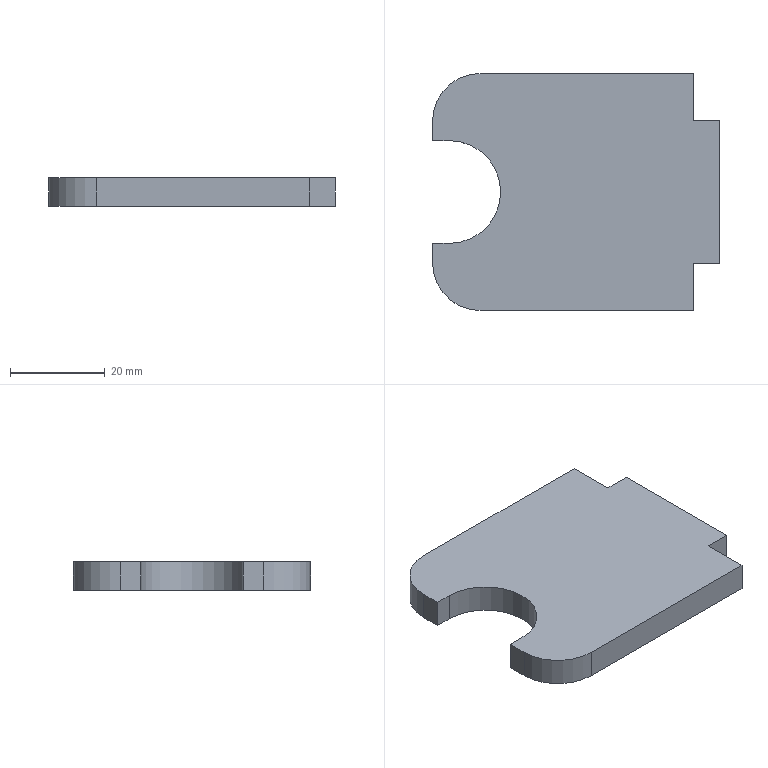Part | SolidWorks | features FlatPattern 1, SMBaseFlange 1, SheetMetal 1 | 1 solid | 16 faces | box 60.5 x 50 x 6 mm | volume 15667 mm3 | plane 13 | cylinder 3 | commonest cylinder face diameters 20 x2 21.7 x1
STEP:
#1=CARTESIAN_POINT('',(-93.75,45.198,0.));
#2=VERTEX_POINT('',#1);
#3=CARTESIAN_POINT('',(-93.75,23.498,0.));
#4=VERTEX_POINT('',#3);
#5=CARTESIAN_POINT('',(-93.75,34.348,0.));
#6=DIRECTION('',(0.,0.,-1.));
#7=DIRECTION('',(1.,0.,0.));
#8=AXIS2_PLACEMENT_3D('',#5,#6,#7);
#9=CIRCLE('',#8,10.85);
#10=EDGE_CURVE('',#2,#4,#9,.T.);
#11=ORIENTED_EDGE('',*,*,#10,.T.);
#12=CARTESIAN_POINT('',(-93.75,23.498,6.));
#13=VERTEX_POINT('',#12);
#14=CARTESIAN_POINT('',(-93.75,23.498,6.));
#15=DIRECTION('',(0.,0.,-1.));
#16=VECTOR('',#15,1000.);
#17=LINE('',#14,#16);
#18=EDGE_CURVE('',#13,#4,#17,.T.);
#19=ORIENTED_EDGE('',*,*,#18,.F.);
#20=CARTESIAN_POINT('',(-93.75,45.198,6.));
#21=VERTEX_POINT('',#20);
#22=CARTESIAN_POINT('',(-93.75,34.348,6.));
#23=DIRECTION('',(0.,0.,-1.));
#24=DIRECTION('',(1.,0.,0.));
#25=AXIS2_PLACEMENT_3D('',#22,#23,#24);
#26=CIRCLE('',#25,10.85);
#27=EDGE_CURVE('',#21,#13,#26,.T.);
#28=ORIENTED_EDGE('',*,*,#27,.F.);
#29=CARTESIAN_POINT('',(-93.75,45.198,6.));
#30=DIRECTION('',(0.,0.,-1.));
#31=VECTOR('',#30,1000.);
#32=LINE('',#29,#31);
#33=EDGE_CURVE('',#21,#2,#32,.T.);
#34=ORIENTED_EDGE('',*,*,#33,.T.);
#35=EDGE_LOOP('',(#11,#19,#28,#34));
#36=FACE_OUTER_BOUND('',#35,.T.);
#37=CARTESIAN_POINT('',(-93.75,34.348,6.));
#38=DIRECTION('',(0.,0.,-1.));
#39=DIRECTION('',(-1.,0.,0.));
#40=AXIS2_PLACEMENT_3D('',#37,#38,#39);
#41=CYLINDRICAL_SURFACE('',#40,10.85);
#42=ADVANCED_FACE('',(#36),#41,.F.);
#43=CARTESIAN_POINT('',(-97.25,23.498,0.));
#44=VERTEX_POINT('',#43);
#45=CARTESIAN_POINT('',(-93.75,23.498,0.));
#46=DIRECTION('',(-1.,0.,0.));
#47=VECTOR('',#46,1000.);
#48=LINE('',#45,#47);
#49=EDGE_CURVE('',#4,#44,#48,.T.);
#50=ORIENTED_EDGE('',*,*,#49,.T.);
#51=CARTESIAN_POINT('',(-97.25,23.498,6.));
#52=VERTEX_POINT('',#51);
#53=CARTESIAN_POINT('',(-97.25,23.498,6.));
#54=DIRECTION('',(0.,0.,-1.));
#55=VECTOR('',#54,1000.);
#56=LINE('',#53,#55);
#57=EDGE_CURVE('',#52,#44,#56,.T.);
#58=ORIENTED_EDGE('',*,*,#57,.F.);
#59=CARTESIAN_POINT('',(-93.75,23.498,6.));
#60=DIRECTION('',(-1.,0.,0.));
#61=VECTOR('',#60,1000.);
#62=LINE('',#59,#61);
#63=EDGE_CURVE('',#13,#52,#62,.T.);
#64=ORIENTED_EDGE('',*,*,#63,.F.);
#65=ORIENTED_EDGE('',*,*,#18,.T.);
#66=EDGE_LOOP('',(#50,#58,#64,#65));
#67=FACE_OUTER_BOUND('',#66,.T.);
#68=CARTESIAN_POINT('',(-93.75,23.498,6.));
#69=DIRECTION('',(0.,-1.,0.));
#70=DIRECTION('',(0.,0.,-1.));
#71=AXIS2_PLACEMENT_3D('',#68,#69,#70);
#72=PLANE('',#71);
#73=ADVANCED_FACE('',(#67),#72,.F.);
#74=CARTESIAN_POINT('',(-97.25,19.348,0.));
#75=VERTEX_POINT('',#74);
#76=CARTESIAN_POINT('',(-97.25,23.498,0.));
#77=DIRECTION('',(0.,-1.,0.));
#78=VECTOR('',#77,1000.);
#79=LINE('',#76,#78);
#80=EDGE_CURVE('',#44,#75,#79,.T.);
#81=ORIENTED_EDGE('',*,*,#80,.T.);
#82=CARTESIAN_POINT('',(-97.25,19.348,6.));
#83=VERTEX_POINT('',#82);
#84=CARTESIAN_POINT('',(-97.25,19.348,6.));
#85=DIRECTION('',(0.,0.,-1.));
#86=VECTOR('',#85,1000.);
#87=LINE('',#84,#86);
#88=EDGE_CURVE('',#83,#75,#87,.T.);
#89=ORIENTED_EDGE('',*,*,#88,.F.);
#90=CARTESIAN_POINT('',(-97.25,23.498,6.));
#91=DIRECTION('',(0.,-1.,0.));
#92=VECTOR('',#91,1000.);
#93=LINE('',#90,#92);
#94=EDGE_CURVE('',#52,#83,#93,.T.);
#95=ORIENTED_EDGE('',*,*,#94,.F.);
#96=ORIENTED_EDGE('',*,*,#57,.T.);
#97=EDGE_LOOP('',(#81,#89,#95,#96));
#98=FACE_OUTER_BOUND('',#97,.T.);
#99=CARTESIAN_POINT('',(-97.25,23.498,6.));
#100=DIRECTION('',(1.,0.,0.));
#101=DIRECTION('',(0.,1.,0.));
#102=AXIS2_PLACEMENT_3D('',#99,#100,#101);
#103=PLANE('',#102);
#104=ADVANCED_FACE('',(#98),#103,.F.);
#105=CARTESIAN_POINT('',(-87.25,9.348,0.));
#106=VERTEX_POINT('',#105);
#107=CARTESIAN_POINT('',(-87.25,19.348,0.));
#108=DIRECTION('',(0.,0.,1.));
#109=DIRECTION('',(1.,0.,0.));
#110=AXIS2_PLACEMENT_3D('',#107,#108,#109);
#111=CIRCLE('',#110,10.);
#112=EDGE_CURVE('',#75,#106,#111,.T.);
#113=ORIENTED_EDGE('',*,*,#112,.T.);
#114=CARTESIAN_POINT('',(-87.25,9.348,6.));
#115=VERTEX_POINT('',#114);
#116=CARTESIAN_POINT('',(-87.25,9.348,6.));
#117=DIRECTION('',(0.,0.,-1.));
#118=VECTOR('',#117,1000.);
#119=LINE('',#116,#118);
#120=EDGE_CURVE('',#115,#106,#119,.T.);
#121=ORIENTED_EDGE('',*,*,#120,.F.);
#122=CARTESIAN_POINT('',(-87.25,19.348,6.));
#123=DIRECTION('',(0.,0.,1.));
#124=DIRECTION('',(1.,0.,0.));
#125=AXIS2_PLACEMENT_3D('',#122,#123,#124);
#126=CIRCLE('',#125,10.);
#127=EDGE_CURVE('',#83,#115,#126,.T.);
#128=ORIENTED_EDGE('',*,*,#127,.F.);
#129=ORIENTED_EDGE('',*,*,#88,.T.);
#130=EDGE_LOOP('',(#113,#121,#128,#129));
#131=FACE_OUTER_BOUND('',#130,.T.);
#132=CARTESIAN_POINT('',(-87.25,19.348,6.));
#133=DIRECTION('',(0.,0.,-1.));
#134=DIRECTION('',(-1.,0.,0.));
#135=AXIS2_PLACEMENT_3D('',#132,#133,#134);
#136=CYLINDRICAL_SURFACE('',#135,10.);
#137=ADVANCED_FACE('',(#131),#136,.T.);
#138=CARTESIAN_POINT('',(-42.25,9.348,0.));
#139=VERTEX_POINT('',#138);
#140=CARTESIAN_POINT('',(-87.25,9.348,0.));
#141=DIRECTION('',(1.,0.,0.));
#142=VECTOR('',#141,1000.);
#143=LINE('',#140,#142);
#144=EDGE_CURVE('',#106,#139,#143,.T.);
#145=ORIENTED_EDGE('',*,*,#144,.T.);
#146=CARTESIAN_POINT('',(-42.25,9.348,6.));
#147=VERTEX_POINT('',#146);
#148=CARTESIAN_POINT('',(-42.25,9.348,6.));
#149=DIRECTION('',(0.,0.,-1.));
#150=VECTOR('',#149,1000.);
#151=LINE('',#148,#150);
#152=EDGE_CURVE('',#147,#139,#151,.T.);
#153=ORIENTED_EDGE('',*,*,#152,.F.);
#154=CARTESIAN_POINT('',(-87.25,9.348,6.));
#155=DIRECTION('',(1.,0.,0.));
#156=VECTOR('',#155,1000.);
#157=LINE('',#154,#156);
#158=EDGE_CURVE('',#115,#147,#157,.T.);
#159=ORIENTED_EDGE('',*,*,#158,.F.);
#160=ORIENTED_EDGE('',*,*,#120,.T.);
#161=EDGE_LOOP('',(#145,#153,#159,#160));
#162=FACE_OUTER_BOUND('',#161,.T.);
#163=CARTESIAN_POINT('',(-87.25,9.348,6.));
#164=DIRECTION('',(0.,1.,0.));
#165=DIRECTION('',(-1.,0.,0.));
#166=AXIS2_PLACEMENT_3D('',#163,#164,#165);
#167=PLANE('',#166);
#168=ADVANCED_FACE('',(#162),#167,.F.);
#169=CARTESIAN_POINT('',(-42.25,19.348,0.));
#170=VERTEX_POINT('',#169);
#171=CARTESIAN_POINT('',(-42.25,9.348,0.));
#172=DIRECTION('',(0.,1.,0.));
#173=VECTOR('',#172,1000.);
#174=LINE('',#171,#173);
#175=EDGE_CURVE('',#139,#170,#174,.T.);
#176=ORIENTED_EDGE('',*,*,#175,.T.);
#177=CARTESIAN_POINT('',(-42.25,19.348,6.));
#178=VERTEX_POINT('',#177);
#179=CARTESIAN_POINT('',(-42.25,19.348,6.));
#180=DIRECTION('',(0.,0.,-1.));
#181=VECTOR('',#180,1000.);
#182=LINE('',#179,#181);
#183=EDGE_CURVE('',#178,#170,#182,.T.);
#184=ORIENTED_EDGE('',*,*,#183,.F.);
#185=CARTESIAN_POINT('',(-42.25,9.348,6.));
#186=DIRECTION('',(0.,1.,0.));
#187=VECTOR('',#186,1000.);
#188=LINE('',#185,#187);
#189=EDGE_CURVE('',#147,#178,#188,.T.);
#190=ORIENTED_EDGE('',*,*,#189,.F.);
#191=ORIENTED_EDGE('',*,*,#152,.T.);
#192=EDGE_LOOP('',(#176,#184,#190,#191));
#193=FACE_OUTER_BOUND('',#192,.T.);
#194=CARTESIAN_POINT('',(-42.25,9.348,6.));
#195=DIRECTION('',(-1.,0.,0.));
#196=DIRECTION('',(0.,0.,1.));
#197=AXIS2_PLACEMENT_3D('',#194,#195,#196);
#198=PLANE('',#197);
#199=ADVANCED_FACE('',(#193),#198,.F.);
#200=CARTESIAN_POINT('',(-36.75,19.348,0.));
#201=VERTEX_POINT('',#200);
#202=CARTESIAN_POINT('',(-42.25,19.348,0.));
#203=DIRECTION('',(1.,0.,0.));
#204=VECTOR('',#203,1000.);
#205=LINE('',#202,#204);
#206=EDGE_CURVE('',#170,#201,#205,.T.);
#207=ORIENTED_EDGE('',*,*,#206,.T.);
#208=CARTESIAN_POINT('',(-36.75,19.348,6.));
#209=VERTEX_POINT('',#208);
#210=CARTESIAN_POINT('',(-36.75,19.348,6.));
#211=DIRECTION('',(0.,0.,-1.));
#212=VECTOR('',#211,1000.);
#213=LINE('',#210,#212);
#214=EDGE_CURVE('',#209,#201,#213,.T.);
#215=ORIENTED_EDGE('',*,*,#214,.F.);
#216=CARTESIAN_POINT('',(-42.25,19.348,6.));
#217=DIRECTION('',(1.,0.,0.));
#218=VECTOR('',#217,1000.);
#219=LINE('',#216,#218);
#220=EDGE_CURVE('',#178,#209,#219,.T.);
#221=ORIENTED_EDGE('',*,*,#220,.F.);
#222=ORIENTED_EDGE('',*,*,#183,.T.);
#223=EDGE_LOOP('',(#207,#215,#221,#222));
#224=FACE_OUTER_BOUND('',#223,.T.);
#225=CARTESIAN_POINT('',(-42.25,19.348,6.));
#226=DIRECTION('',(0.,1.,0.));
#227=DIRECTION('',(-1.,0.,0.));
#228=AXIS2_PLACEMENT_3D('',#225,#226,#227);
#229=PLANE('',#228);
#230=ADVANCED_FACE('',(#224),#229,.F.);
#231=CARTESIAN_POINT('',(-36.75,49.348,0.));
#232=VERTEX_POINT('',#231);
#233=CARTESIAN_POINT('',(-36.75,19.348,0.));
#234=DIRECTION('',(0.,1.,0.));
#235=VECTOR('',#234,1000.);
#236=LINE('',#233,#235);
#237=EDGE_CURVE('',#201,#232,#236,.T.);
#238=ORIENTED_EDGE('',*,*,#237,.T.);
#239=CARTESIAN_POINT('',(-36.75,49.348,6.));
#240=VERTEX_POINT('',#239);
#241=CARTESIAN_POINT('',(-36.75,49.348,6.));
#242=DIRECTION('',(0.,0.,-1.));
#243=VECTOR('',#242,1000.);
#244=LINE('',#241,#243);
#245=EDGE_CURVE('',#240,#232,#244,.T.);
#246=ORIENTED_EDGE('',*,*,#245,.F.);
#247=CARTESIAN_POINT('',(-36.75,19.348,6.));
#248=DIRECTION('',(0.,1.,0.));
#249=VECTOR('',#248,1000.);
#250=LINE('',#247,#249);
#251=EDGE_CURVE('',#209,#240,#250,.T.);
#252=ORIENTED_EDGE('',*,*,#251,.F.);
#253=ORIENTED_EDGE('',*,*,#214,.T.);
#254=EDGE_LOOP('',(#238,#246,#252,#253));
#255=FACE_OUTER_BOUND('',#254,.T.);
#256=CARTESIAN_POINT('',(-36.75,19.348,6.));
#257=DIRECTION('',(-1.,0.,0.));
#258=DIRECTION('',(0.,0.,1.));
#259=AXIS2_PLACEMENT_3D('',#256,#257,#258);
#260=PLANE('',#259);
#261=ADVANCED_FACE('',(#255),#260,.F.);
#262=CARTESIAN_POINT('',(-42.25,49.348,0.));
#263=VERTEX_POINT('',#262);
#264=CARTESIAN_POINT('',(-36.75,49.348,0.));
#265=DIRECTION('',(-1.,0.,0.));
#266=VECTOR('',#265,1000.);
#267=LINE('',#264,#266);
#268=EDGE_CURVE('',#232,#263,#267,.T.);
#269=ORIENTED_EDGE('',*,*,#268,.T.);
#270=CARTESIAN_POINT('',(-42.25,49.348,6.));
#271=VERTEX_POINT('',#270);
#272=CARTESIAN_POINT('',(-42.25,49.348,6.));
#273=DIRECTION('',(0.,0.,-1.));
#274=VECTOR('',#273,1000.);
#275=LINE('',#272,#274);
#276=EDGE_CURVE('',#271,#263,#275,.T.);
#277=ORIENTED_EDGE('',*,*,#276,.F.);
#278=CARTESIAN_POINT('',(-36.75,49.348,6.));
#279=DIRECTION('',(-1.,0.,0.));
#280=VECTOR('',#279,1000.);
#281=LINE('',#278,#280);
#282=EDGE_CURVE('',#240,#271,#281,.T.);
#283=ORIENTED_EDGE('',*,*,#282,.F.);
#284=ORIENTED_EDGE('',*,*,#245,.T.);
#285=EDGE_LOOP('',(#269,#277,#283,#284));
#286=FACE_OUTER_BOUND('',#285,.T.);
#287=CARTESIAN_POINT('',(-36.75,49.348,6.));
#288=DIRECTION('',(0.,-1.,0.));
#289=DIRECTION('',(1.,0.,0.));
#290=AXIS2_PLACEMENT_3D('',#287,#288,#289);
#291=PLANE('',#290);
#292=ADVANCED_FACE('',(#286),#291,.F.);
#293=CARTESIAN_POINT('',(-42.25,59.348,0.));
#294=VERTEX_POINT('',#293);
#295=CARTESIAN_POINT('',(-42.25,49.348,0.));
#296=DIRECTION('',(0.,1.,0.));
#297=VECTOR('',#296,1000.);
#298=LINE('',#295,#297);
#299=EDGE_CURVE('',#263,#294,#298,.T.);
#300=ORIENTED_EDGE('',*,*,#299,.T.);
#301=CARTESIAN_POINT('',(-42.25,59.348,6.));
#302=VERTEX_POINT('',#301);
#303=CARTESIAN_POINT('',(-42.25,59.348,6.));
#304=DIRECTION('',(0.,0.,-1.));
#305=VECTOR('',#304,1000.);
#306=LINE('',#303,#305);
#307=EDGE_CURVE('',#302,#294,#306,.T.);
#308=ORIENTED_EDGE('',*,*,#307,.F.);
#309=CARTESIAN_POINT('',(-42.25,49.348,6.));
#310=DIRECTION('',(0.,1.,0.));
#311=VECTOR('',#310,1000.);
#312=LINE('',#309,#311);
#313=EDGE_CURVE('',#271,#302,#312,.T.);
#314=ORIENTED_EDGE('',*,*,#313,.F.);
#315=ORIENTED_EDGE('',*,*,#276,.T.);
#316=EDGE_LOOP('',(#300,#308,#314,#315));
#317=FACE_OUTER_BOUND('',#316,.T.);
#318=CARTESIAN_POINT('',(-42.25,49.348,6.));
#319=DIRECTION('',(-1.,0.,0.));
#320=DIRECTION('',(0.,0.,1.));
#321=AXIS2_PLACEMENT_3D('',#318,#319,#320);
#322=PLANE('',#321);
#323=ADVANCED_FACE('',(#317),#322,.F.);
#324=CARTESIAN_POINT('',(-87.25,59.348,0.));
#325=VERTEX_POINT('',#324);
#326=CARTESIAN_POINT('',(-87.25,59.348,0.));
#327=DIRECTION('',(-1.,0.,0.));
#328=VECTOR('',#327,1000.);
#329=LINE('',#326,#328);
#330=EDGE_CURVE('',#294,#325,#329,.T.);
#331=ORIENTED_EDGE('',*,*,#330,.T.);
#332=CARTESIAN_POINT('',(-87.25,59.348,6.));
#333=VERTEX_POINT('',#332);
#334=CARTESIAN_POINT('',(-87.25,59.348,6.));
#335=DIRECTION('',(0.,0.,-1.));
#336=VECTOR('',#335,1000.);
#337=LINE('',#334,#336);
#338=EDGE_CURVE('',#333,#325,#337,.T.);
#339=ORIENTED_EDGE('',*,*,#338,.F.);
#340=CARTESIAN_POINT('',(-87.25,59.348,6.));
#341=DIRECTION('',(-1.,0.,0.));
#342=VECTOR('',#341,1000.);
#343=LINE('',#340,#342);
#344=EDGE_CURVE('',#302,#333,#343,.T.);
#345=ORIENTED_EDGE('',*,*,#344,.F.);
#346=ORIENTED_EDGE('',*,*,#307,.T.);
#347=EDGE_LOOP('',(#331,#339,#345,#346));
#348=FACE_OUTER_BOUND('',#347,.T.);
#349=CARTESIAN_POINT('',(-87.25,59.348,6.));
#350=DIRECTION('',(0.,-1.,0.));
#351=DIRECTION('',(0.,0.,-1.));
#352=AXIS2_PLACEMENT_3D('',#349,#350,#351);
#353=PLANE('',#352);
#354=ADVANCED_FACE('',(#348),#353,.F.);
#355=CARTESIAN_POINT('',(-97.25,49.348,0.));
#356=VERTEX_POINT('',#355);
#357=CARTESIAN_POINT('',(-87.25,49.348,0.));
#358=DIRECTION('',(0.,0.,1.));
#359=DIRECTION('',(-1.,0.,0.));
#360=AXIS2_PLACEMENT_3D('',#357,#358,#359);
#361=CIRCLE('',#360,10.);
#362=EDGE_CURVE('',#325,#356,#361,.T.);
#363=ORIENTED_EDGE('',*,*,#362,.T.);
#364=CARTESIAN_POINT('',(-97.25,49.348,6.));
#365=VERTEX_POINT('',#364);
#366=CARTESIAN_POINT('',(-97.25,49.348,6.));
#367=DIRECTION('',(0.,0.,-1.));
#368=VECTOR('',#367,1000.);
#369=LINE('',#366,#368);
#370=EDGE_CURVE('',#365,#356,#369,.T.);
#371=ORIENTED_EDGE('',*,*,#370,.F.);
#372=CARTESIAN_POINT('',(-87.25,49.348,6.));
#373=DIRECTION('',(0.,0.,1.));
#374=DIRECTION('',(-1.,0.,0.));
#375=AXIS2_PLACEMENT_3D('',#372,#373,#374);
#376=CIRCLE('',#375,10.);
#377=EDGE_CURVE('',#333,#365,#376,.T.);
#378=ORIENTED_EDGE('',*,*,#377,.F.);
#379=ORIENTED_EDGE('',*,*,#338,.T.);
#380=EDGE_LOOP('',(#363,#371,#378,#379));
#381=FACE_OUTER_BOUND('',#380,.T.);
#382=CARTESIAN_POINT('',(-87.25,49.348,6.));
#383=DIRECTION('',(0.,0.,-1.));
#384=DIRECTION('',(-1.,0.,0.));
#385=AXIS2_PLACEMENT_3D('',#382,#383,#384);
#386=CYLINDRICAL_SURFACE('',#385,10.);
#387=ADVANCED_FACE('',(#381),#386,.T.);
#388=CARTESIAN_POINT('',(-97.25,45.198,0.));
#389=VERTEX_POINT('',#388);
#390=CARTESIAN_POINT('',(-97.25,45.198,0.));
#391=DIRECTION('',(0.,-1.,0.));
#392=VECTOR('',#391,1000.);
#393=LINE('',#390,#392);
#394=EDGE_CURVE('',#356,#389,#393,.T.);
#395=ORIENTED_EDGE('',*,*,#394,.T.);
#396=CARTESIAN_POINT('',(-97.25,45.198,6.));
#397=VERTEX_POINT('',#396);
#398=CARTESIAN_POINT('',(-97.25,45.198,6.));
#399=DIRECTION('',(0.,0.,-1.));
#400=VECTOR('',#399,1000.);
#401=LINE('',#398,#400);
#402=EDGE_CURVE('',#397,#389,#401,.T.);
#403=ORIENTED_EDGE('',*,*,#402,.F.);
#404=CARTESIAN_POINT('',(-97.25,45.198,6.));
#405=DIRECTION('',(0.,-1.,0.));
#406=VECTOR('',#405,1000.);
#407=LINE('',#404,#406);
#408=EDGE_CURVE('',#365,#397,#407,.T.);
#409=ORIENTED_EDGE('',*,*,#408,.F.);
#410=ORIENTED_EDGE('',*,*,#370,.T.);
#411=EDGE_LOOP('',(#395,#403,#409,#410));
#412=FACE_OUTER_BOUND('',#411,.T.);
#413=CARTESIAN_POINT('',(-97.25,45.198,6.));
#414=DIRECTION('',(1.,0.,0.));
#415=DIRECTION('',(0.,1.,0.));
#416=AXIS2_PLACEMENT_3D('',#413,#414,#415);
#417=PLANE('',#416);
#418=ADVANCED_FACE('',(#412),#417,.F.);
#419=CARTESIAN_POINT('',(-93.75,45.198,0.));
#420=DIRECTION('',(1.,0.,0.));
#421=VECTOR('',#420,1000.);
#422=LINE('',#419,#421);
#423=EDGE_CURVE('',#389,#2,#422,.T.);
#424=ORIENTED_EDGE('',*,*,#423,.T.);
#425=ORIENTED_EDGE('',*,*,#33,.F.);
#426=CARTESIAN_POINT('',(-93.75,45.198,6.));
#427=DIRECTION('',(1.,0.,0.));
#428=VECTOR('',#427,1000.);
#429=LINE('',#426,#428);
#430=EDGE_CURVE('',#397,#21,#429,.T.);
#431=ORIENTED_EDGE('',*,*,#430,.F.);
#432=ORIENTED_EDGE('',*,*,#402,.T.);
#433=EDGE_LOOP('',(#424,#425,#431,#432));
#434=FACE_OUTER_BOUND('',#433,.T.);
#435=CARTESIAN_POINT('',(-93.75,45.198,6.));
#436=DIRECTION('',(0.,1.,0.));
#437=DIRECTION('',(0.,0.,1.));
#438=AXIS2_PLACEMENT_3D('',#435,#436,#437);
#439=PLANE('',#438);
#440=ADVANCED_FACE('',(#434),#439,.F.);
#441=ORIENTED_EDGE('',*,*,#27,.T.);
#442=ORIENTED_EDGE('',*,*,#63,.T.);
#443=ORIENTED_EDGE('',*,*,#94,.T.);
#444=ORIENTED_EDGE('',*,*,#127,.T.);
#445=ORIENTED_EDGE('',*,*,#158,.T.);
#446=ORIENTED_EDGE('',*,*,#189,.T.);
#447=ORIENTED_EDGE('',*,*,#220,.T.);
#448=ORIENTED_EDGE('',*,*,#251,.T.);
#449=ORIENTED_EDGE('',*,*,#282,.T.);
#450=ORIENTED_EDGE('',*,*,#313,.T.);
#451=ORIENTED_EDGE('',*,*,#344,.T.);
#452=ORIENTED_EDGE('',*,*,#377,.T.);
#453=ORIENTED_EDGE('',*,*,#408,.T.);
#454=ORIENTED_EDGE('',*,*,#430,.T.);
#455=EDGE_LOOP('',(#441,#442,#443,#444,#445,#446,#447,#448,#449,#450,#451,#452,#453,#454));
#456=FACE_OUTER_BOUND('',#455,.T.);
#457=CARTESIAN_POINT('',(-93.75,34.348,6.));
#458=DIRECTION('',(0.,0.,1.));
#459=DIRECTION('',(1.,0.,0.));
#460=AXIS2_PLACEMENT_3D('',#457,#458,#459);
#461=PLANE('',#460);
#462=ADVANCED_FACE('',(#456),#461,.T.);
#463=ORIENTED_EDGE('',*,*,#10,.F.);
#464=ORIENTED_EDGE('',*,*,#423,.F.);
#465=ORIENTED_EDGE('',*,*,#394,.F.);
#466=ORIENTED_EDGE('',*,*,#362,.F.);
#467=ORIENTED_EDGE('',*,*,#330,.F.);
#468=ORIENTED_EDGE('',*,*,#299,.F.);
#469=ORIENTED_EDGE('',*,*,#268,.F.);
#470=ORIENTED_EDGE('',*,*,#237,.F.);
#471=ORIENTED_EDGE('',*,*,#206,.F.);
#472=ORIENTED_EDGE('',*,*,#175,.F.);
#473=ORIENTED_EDGE('',*,*,#144,.F.);
#474=ORIENTED_EDGE('',*,*,#112,.F.);
#475=ORIENTED_EDGE('',*,*,#80,.F.);
#476=ORIENTED_EDGE('',*,*,#49,.F.);
#477=EDGE_LOOP('',(#463,#464,#465,#466,#467,#468,#469,#470,#471,#472,#473,#474,#475,#476));
#478=FACE_OUTER_BOUND('',#477,.T.);
#479=CARTESIAN_POINT('',(-93.75,34.348,0.));
#480=DIRECTION('',(0.,0.,1.));
#481=DIRECTION('',(1.,0.,0.));
#482=AXIS2_PLACEMENT_3D('',#479,#480,#481);
#483=PLANE('',#482);
#484=ADVANCED_FACE('',(#478),#483,.F.);
#485=CLOSED_SHELL('',(#42,#73,#104,#137,#168,#199,#230,#261,#292,#323,#354,#387,#418,#440,#462,#484));
#486=MANIFOLD_SOLID_BREP('',#485);
#487=CARTESIAN_POINT('',(0.,0.,0.));
#488=DIRECTION('',(0.,0.,1.));
#489=DIRECTION('',(1.,0.,0.));
#490=AXIS2_PLACEMENT_3D('',#487,#488,#489);
#491=(LENGTH_UNIT()NAMED_UNIT(*)SI_UNIT(.MILLI.,.METRE.));
#492=UNCERTAINTY_MEASURE_WITH_UNIT(LENGTH_MEASURE(0.00001),#491,'','');
#493=(NAMED_UNIT(*)PLANE_ANGLE_UNIT()SI_UNIT($,.RADIAN.));
#494=(NAMED_UNIT(*)SI_UNIT($,.STERADIAN.)SOLID_ANGLE_UNIT());
#495=(GEOMETRIC_REPRESENTATION_CONTEXT(3)GLOBAL_UNCERTAINTY_ASSIGNED_CONTEXT((#492))GLOBAL_UNIT_ASSIGNED_CONTEXT((#491,#493,#494))REPRESENTATION_CONTEXT('',''));
#496=ADVANCED_BREP_SHAPE_REPRESENTATION('',(#486,#490),#495);